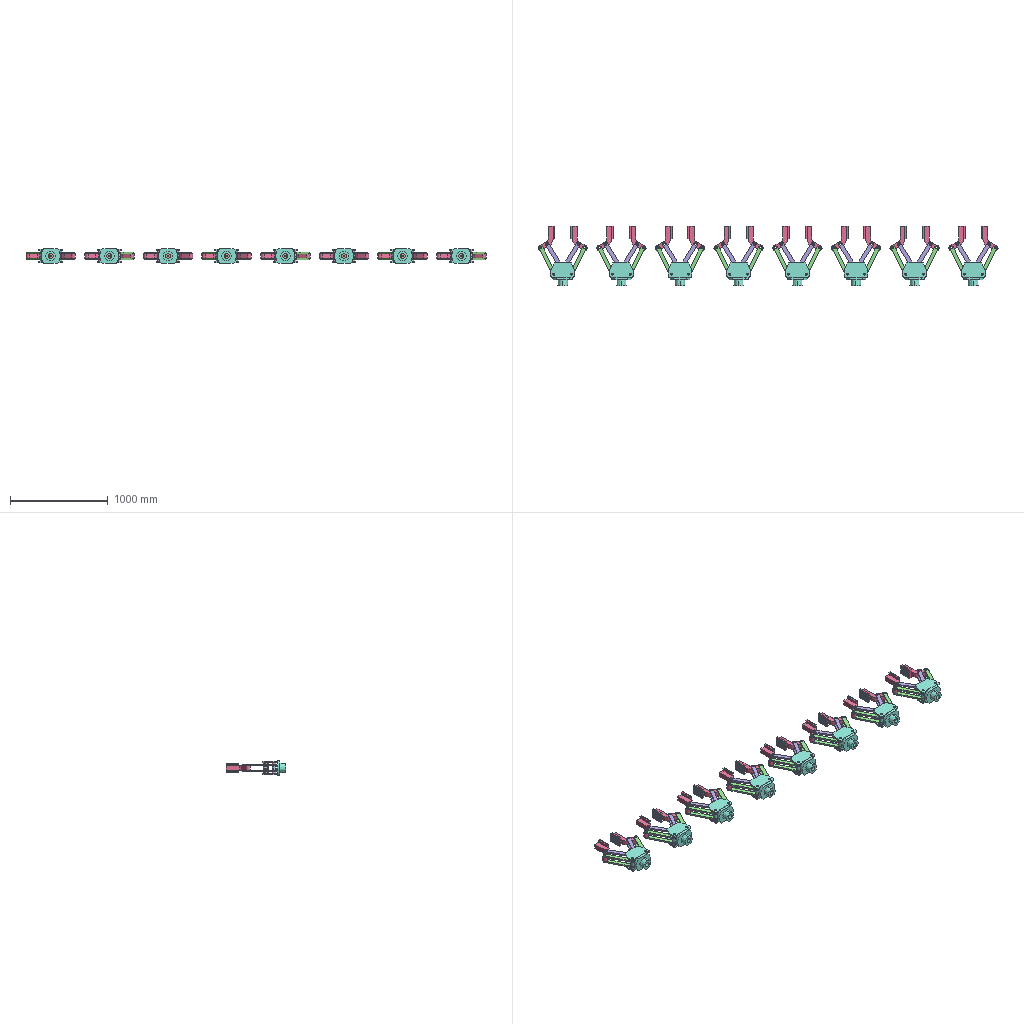Assembly | SolidWorks | 6 different items | 128 placed | box 4705 x 610 x 150 mm
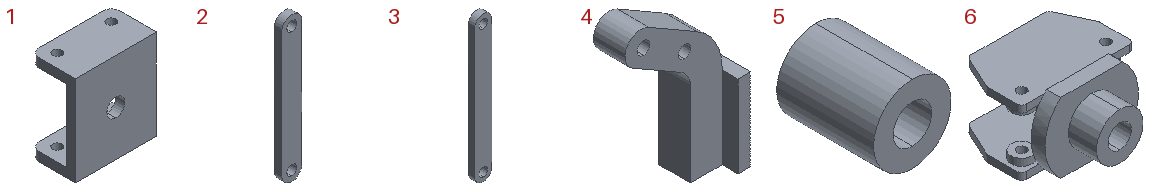Parts list (item | quantity | size | volume | features):
1 | x8 | 90 x 50 x 100 mm | 154858 mm3 | features ICE 4, MoveFace 4, Extrusion 1, Fillet 1
2 | x32 | 40 x 15 x 290 mm | 159425 mm3 | features Extrusion 1
3 | x32 | 40 x 15 x 340 mm | 189425 mm3 | features Extrusion 1
4 | x16 | 173.433 x 100 x 249.151 mm | 959009 mm3 | features ICE 2, Extrusion 1, Fillet 1
5 | x32 | 40 x 50 x 40 mm | 47124 mm3 | features Extrusion 1
6 | x8 | 240 x 240 x 150 mm | 2158258 mm3 | features ICE 9, Fillet 2, Extrusion 1
Mates (type | each side: item.copy, entity, surface, feature):
Concentric | 6.1 face cylinder Cut-Extrude3 | 1.1 face cylinder Cut-Extrude4
Parallel | 6.1 face plane Boss-Extrude3 | 1.1 face plane Boss-Extrude1
Concentric | 1.1 face cylinder Cut-Extrude3 | 2.1 face cylinder Boss-Extrude1
Coincident | 1.1 face plane Cut-Extrude1 | 2.1 face plane Boss-Extrude1
Concentric | 6.1 face cylinder Cut-Extrude4 | 3.1 face cylinder Boss-Extrude1
Coincident | 6.1 face plane Boss-Extrude5 | 3.1 face plane Boss-Extrude1
Concentric | 1.1 face cylinder Cut-Extrude3 | 2.2 face cylinder Boss-Extrude1
Coincident | 1.1 face plane Cut-Extrude1 | 2.2 face plane Boss-Extrude1
Concentric | 6.1 face cylinder Boss-Extrude5 | 3.2 face cylinder Boss-Extrude1
Coincident | 6.1 face plane Boss-Extrude4 | 3.2 face plane Boss-Extrude1
Coincident | 3.1 face plane Boss-Extrude1 | 4.1 face plane Boss-Extrude1
Concentric | 3.1 face cylinder Boss-Extrude1 | 4.1 face cylinder Boss-Extrude1
Concentric | 2.1 face cylinder Boss-Extrude1 | 4.1 face cylinder Boss-Extrude1
Concentric | 3.2 face cylinder Boss-Extrude1 | 4.2 face cylinder Boss-Extrude1
Concentric | 6.1 face cylinder Boss-Extrude4 | 3.3 face cylinder Boss-Extrude1
Coincident | 6.1 face plane Boss-Extrude4 | 3.3 face plane Boss-Extrude1
Coincident | 1.1 face plane Cut-Extrude1 | 2.3 face plane Boss-Extrude1
Concentric | 2.1 face cylinder Boss-Extrude1 | 2.3 face cylinder Boss-Extrude1
Concentric | 2.2 face cylinder Boss-Extrude1 | 4.2 face cylinder Boss-Extrude1
Coincident | 2.2 face plane Boss-Extrude1 | 4.2 face plane Boss-Extrude1
Concentric | 1.1 face cylinder Cut-Extrude3 | 2.4 face cylinder Boss-Extrude1
Coincident | 1.1 face plane Cut-Extrude1 | 2.4 face plane Boss-Extrude1
Concentric | 4.2 face cylinder Boss-Extrude1 | 2.4 face cylinder Boss-Extrude1
Concentric | 6.1 face cylinder Boss-Extrude5 | 3.4 face cylinder Boss-Extrude1
Coincident | 6.1 face plane Boss-Extrude5 | 3.4 face plane Boss-Extrude1
Concentric | 4.2 face cylinder Boss-Extrude1 | 3.4 face cylinder Boss-Extrude1
Concentric | 4.1 face cylinder Boss-Extrude1 | 2.3 face cylinder Boss-Extrude1
Concentric | 4.1 face cylinder Boss-Extrude1 | 3.3 face cylinder Boss-Extrude1
Coincident | 4.1 face plane Boss-Extrude1 | 4.2 face plane Boss-Extrude1
Concentric | 3.1 face cylinder Boss-Extrude1 | 5.1 face cylinder Boss-Extrude1
Coincident | 3.1 face plane Boss-Extrude1 | 5.1 face plane Boss-Extrude1
Concentric | 2.1 face cylinder Boss-Extrude1 | 5.2 face cylinder Boss-Extrude1
Coincident | 2.1 face plane Boss-Extrude1 | 5.2 face plane Boss-Extrude1
Concentric | 2.2 face cylinder Boss-Extrude1 | 5.3 face cylinder Boss-Extrude1
Coincident | 2.2 face plane Boss-Extrude1 | 5.3 face plane Boss-Extrude1
Concentric | 3.4 face cylinder Boss-Extrude1 | 5.4 face cylinder Boss-Extrude1
Coincident | 3.4 face plane Boss-Extrude1 | 5.4 face plane Boss-Extrude1